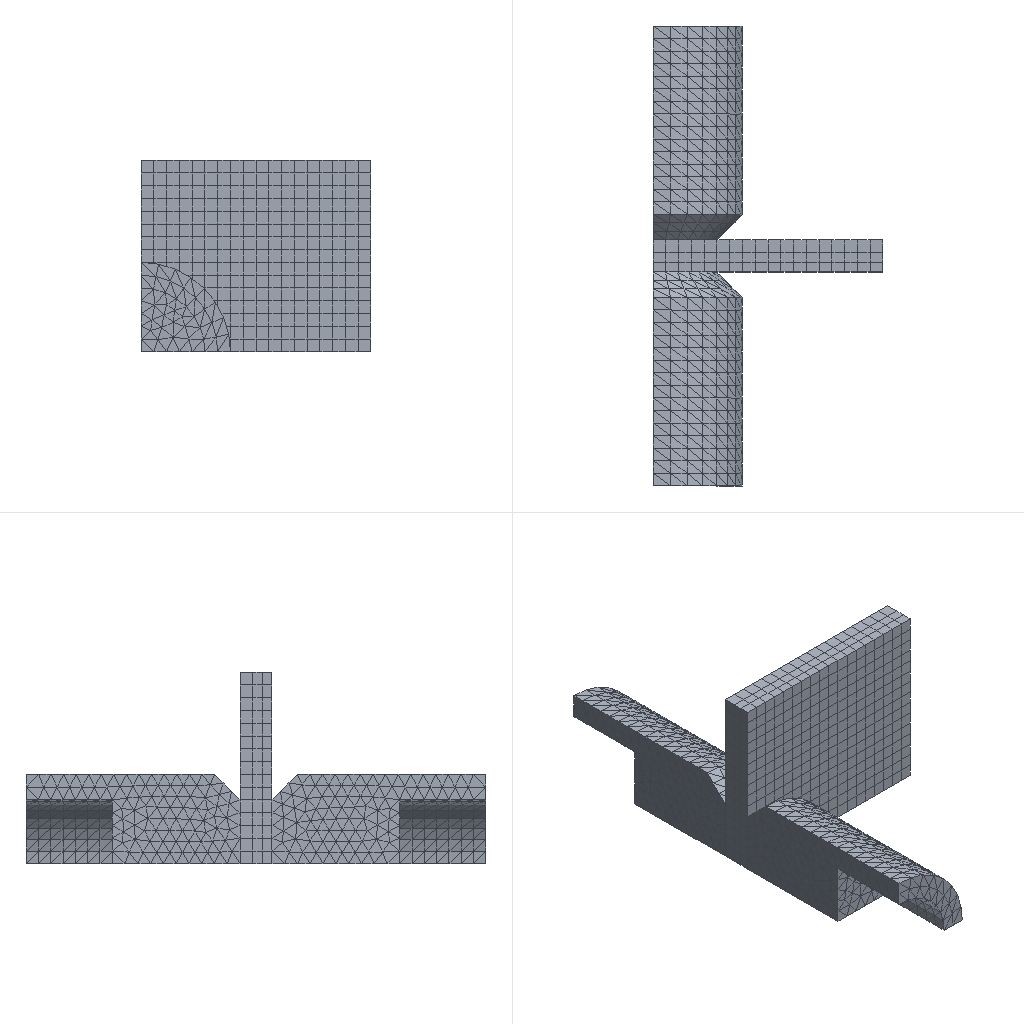Simulation study | abaqus
Set-up summary:
category,name,step,type,value,unit,region
solver,abaqus
solver,version,,,Abaqus/Standard 3DEXPERIENCE R2017x
units,not stated in the deck,,not stated
analysis,deck,,coupled temperature-displacement,coupled temperature-displacement
load_step,Step-1,Step-1,coupled temperature-displacement
load_step,requested,,,1
mesh,nodes,,,3054
mesh,elements,,,7094
element_type,Q3D4,,solid,6284
element_type,Q3D8,,solid,810
load,load commands in deck,,count,3
bc,support commands in deck,,count,5
material,BAN,,in results
material,DIANJI,,in results
check,setup vs results,,match,"per instance, exact: element labels, types and connectivity; labels of the nodes the elements use; coordinates of those nodes at SINGLE_PRECISION in 1 of 4 instance(s)"
Abaqus input file, long lists of numbers shortened:
*Heading
** Job name: Job-1 Model name: Model-1
** Generated by: Abaqus/CAE 2017
*Preprint, echo=NO, model=NO, history=NO, contact=NO
**
** PARTS
**
*Part, name=Part-1
*Node
      1,           0.,          10.,           5.
      2,           0.,        16.75,           5.
** (765 more lines like these left out)
*Element, type=Q3D4
   1, 440, 441, 442, 443
   2, 443, 444, 445, 446
** (3140 more lines like these left out)
*Nset, nset=Set-1, generate
   1,  767,    1
*Elset, elset=Set-1, generate
    1,  3142,     1
** Section: dianji
*Solid Section, elset=Set-1, material=dianji
,
*End Part
**
*Part, name=ban1
*Node
      1,           0.,          -1.,          15.
      2,           0.,           0.,          15.
** (606 more lines like these left out)
*Element, type=Q3D8
  1,  33,  34,  36,  35,   1,   2,   4,   3
  2,  35,  36,  38,  37,   3,   4,   6,   5
** (268 more lines like these left out)
*Nset, nset=Set-1, generate
   1,  608,    1
*Elset, elset=Set-1, generate
   1,  270,    1
** Section: ban
*Solid Section, elset=Set-1, material=ban
,
*End Part
**
*Part, name=ban1point5
*Node
      1,           0.,         -1.5,          15.
      2,           0.,        -0.75,          15.
** (910 more lines like these left out)
*Element, type=Q3D8
  1,  49,  50,  53,  52,   1,   2,   5,   4
  2,  50,  51,  54,  53,   2,   3,   6,   5
** (538 more lines like these left out)
*Nset, nset=Set-1, generate
   1,  912,    1
*Elset, elset=Set-1, generate
   1,  540,    1
** Section: ban
*Solid Section, elset=Set-1, material=ban
,
*End Part
**
**
** ASSEMBLY
**
*Assembly, name=Assembly
**
*Instance, name=Part-1-1, part=Part-1
          0.,           1.,           0.
*End Instance
**
*Instance, name=ban1-1, part=ban1
          0.,           1.,           0.
*End Instance
**
*Instance, name=ban1point5-1, part=ban1point5
*End Instance
**
*Instance, name=Part-1-2, part=Part-1
          0.,         -1.5,           0.
          0.,         -1.5,           0., 0.7071,         -1.5, 0.7071,         180.
*End Instance
**
*Nset, nset=Set-1, instance=Part-1-1, generate
   1,  767,    1
*Nset, nset=Set-1, instance=ban1-1, generate
   1,  608,    1
*Nset, nset=Set-1, instance=Part-1-2, generate
   1,  767,    1
*Nset, nset=Set-1, instance=ban1point5-1, generate
   1,  912,    1
*Elset, elset=Set-1, instance=Part-1-1, generate
    1,  3142,     1
*Elset, elset=Set-1, instance=ban1-1, generate
   1,  270,    1
*Elset, elset=Set-1, instance=Part-1-2, generate
    1,  3142,     1
*Elset, elset=Set-1, instance=ban1point5-1, generate
   1,  540,    1
*Nset, nset=Set-2, instance=Part-1-1
   3,   4,   6,   7,   9,  10,  11,  26,  27,  28,  29,  30,  31,  47,  52,  53
  54,  55,  77,  78,  79,  80,  81,  82,  83,  84,  85,  86,  87,  88,  89,  90
** (6 more lines like these left out)
*Nset, nset=Set-2, instance=ban1point5-1
  46,  47,  48,  94,  95,  96, 142, 143, 144, 190, 191, 192, 238, 239, 240, 286
 287, 288, 334, 335, 336, 382, 383, 384, 430, 431, 432, 478, 479, 480, 526, 527
** (2 more lines like these left out)
*Nset, nset=Set-2, instance=Part-1-2
   1,   2,   5,   7,   8,  10,  12,  13,  14,  15,  16,  17,  18,  39,  48,  49
  50,  51,  56,  57,  58,  59,  60,  61,  62,  63,  64,  65,  66,  67,  68,  69
** (6 more lines like these left out)
*Elset, elset=Set-2, instance=Part-1-1
  116,  177,  264,  308,  314,  315,  320,  363,  385,  387,  416,  469,  470,  471,  567,  570
  572,  573,  577,  593,  610,  628,  638,  657,  724,  725,  748,  755,  778,  785,  788,  801
** (10 more lines like these left out)
*Elset, elset=Set-2, instance=ban1point5-1
  29,  30,  59,  60,  89,  90, 119, 120, 149, 150, 179, 180, 209, 210, 239, 240
 269, 270, 299, 300, 329, 330, 359, 360, 389, 390, 419, 420, 449, 450, 479, 480
** (1 more lines like these left out)
*Elset, elset=Set-2, instance=Part-1-2
  315,  487,  536,  593,  598,  621,  622,  624,  632,  634,  635,  636,  637,  641,  643,  644
  653,  774,  796,  802,  908,  974,  992, 1022, 1123, 1154, 1191, 1193, 1223, 1229, 1233, 1249
** (10 more lines like these left out)
*Nset, nset=Set-3, instance=Part-1-1
   1,   2,   5,   7,   8,  10,  12,  13,  14,  15,  16,  17,  18,  39,  48,  49
  50,  51,  56,  57,  58,  59,  60,  61,  62,  63,  64,  65,  66,  67,  68,  69
** (6 more lines like these left out)
*Nset, nset=Set-3, instance=ban1point5-1, generate
  1,  48,   1
*Nset, nset=Set-3, instance=Part-1-2
   3,   4,   6,   7,   9,  10,  11,  26,  27,  28,  29,  30,  31,  47,  52,  53
  54,  55,  77,  78,  79,  80,  81,  82,  83,  84,  85,  86,  87,  88,  89,  90
** (6 more lines like these left out)
*Elset, elset=Set-3, instance=Part-1-1
  315,  487,  536,  593,  598,  621,  622,  624,  632,  634,  635,  636,  637,  641,  643,  644
  653,  774,  796,  802,  908,  974,  992, 1022, 1123, 1154, 1191, 1193, 1223, 1229, 1233, 1249
** (10 more lines like these left out)
*Elset, elset=Set-3, instance=ban1point5-1, generate
  1,  30,   1
*Elset, elset=Set-3, instance=Part-1-2
  116,  177,  264,  308,  314,  315,  320,  363,  385,  387,  416,  469,  470,  471,  567,  570
  572,  573,  577,  593,  610,  628,  638,  657,  724,  725,  748,  755,  778,  785,  788,  801
** (10 more lines like these left out)
*Nset, nset=Set-4, instance=Part-1-1
   2,   3,   5,   6,  19,  20,  21,  22,  23,  24,  25,  39,  40,  41,  42,  43
  44,  45,  46,  47, 161, 162, 163, 164, 165, 166, 167
*Elset, elset=Set-4, instance=Part-1-1
  277,  488,  757,  763,  764,  784, 1313, 1450, 1600, 1730, 1733, 1829, 1901, 1906, 1926, 2058
 2060, 2062, 2089, 2106, 2123, 2149, 2169, 2172, 2181, 2200, 2268, 2324, 2342, 2391, 2684, 2735
*Nset, nset=Set-5, instance=Part-1-1
   2,   3,   5,   6,  19,  20,  21,  22,  23,  24,  25,  39,  40,  41,  42,  43
  44,  45,  46,  47, 161, 162, 163, 164, 165, 166, 167
*Elset, elset=Set-5, instance=Part-1-1
  277,  488,  757,  763,  764,  784, 1313, 1450, 1600, 1730, 1733, 1829, 1901, 1906, 1926, 2058
 2060, 2062, 2089, 2106, 2123, 2149, 2169, 2172, 2181, 2200, 2268, 2324, 2342, 2391, 2684, 2735
*Elset, elset=_Surf-1_S1, internal, instance=ban1-1, generate
 256,  270,    1
*Elset, elset=_Surf-1_S1, internal, instance=ban1point5-1, generate
 511,  540,    1
*Elset, elset=_Surf-1_S6, internal, instance=ban1-1, generate
   1,  270,    1
*Elset, elset=_Surf-1_S6, internal, instance=ban1point5-1, generate
   1,  539,    2
*Elset, elset=_Surf-1_S2, internal, instance=ban1-1, generate
  1,  15,   1
*Elset, elset=_Surf-1_S2, internal, instance=ban1point5-1, generate
  1,  30,   1
*Elset, elset=_Surf-1_S4, internal, instance=ban1-1, generate
   1,  270,    1
*Elset, elset=_Surf-1_S4, internal, instance=ban1point5-1, generate
   2,  540,    2
*Elset, elset=_Surf-1_S3, internal, instance=ban1-1, generate
   1,  256,   15
*Elset, elset=_Surf-1_S3, internal, instance=ban1point5-1
   1,   2,  31,  32,  61,  62,  91,  92, 121, 122, 151, 152, 181, 182, 211, 212
 241, 242, 271, 272, 301, 302, 331, 332, 361, 362, 391, 392, 421, 422, 451, 452
** (1 more lines like these left out)
*Elset, elset=_Surf-1_S5, internal, instance=ban1-1, generate
  15,  270,   15
*Elset, elset=_Surf-1_S5, internal, instance=ban1point5-1
  29,  30,  59,  60,  89,  90, 119, 120, 149, 150, 179, 180, 209, 210, 239, 240
 269, 270, 299, 300, 329, 330, 359, 360, 389, 390, 419, 420, 449, 450, 479, 480
** (1 more lines like these left out)
*Surface, type=ELEMENT, name=Surf-1
_Surf-1_S1, S1
_Surf-1_S6, S6
_Surf-1_S2, S2
_Surf-1_S4, S4
_Surf-1_S3, S3
_Surf-1_S5, S5
*Elset, elset=_Surf-2_S3, internal, instance=Part-1-2
  277,  488,  757,  763,  764,  784, 1313, 1450, 1600, 1733, 1901, 1906, 2058, 2060, 2062, 2089
 2106, 2149, 2169, 2172, 2181, 2268, 2324, 2391, 2684, 2735
*Elset, elset=_Surf-2_S2, internal, instance=Part-1-2
 1730, 1926
*Elset, elset=_Surf-2_S4, internal, instance=Part-1-2
 1829, 2123
*Elset, elset=_Surf-2_S1, internal, instance=Part-1-2
 2200, 2342
*Surface, type=ELEMENT, name=Surf-2
_Surf-2_S3, S3
_Surf-2_S2, S2
_Surf-2_S4, S4
_Surf-2_S1, S1
*Elset, elset=_Surf-3_S3, internal, instance=Part-1-2
  113,  796, 1579, 1757, 1890, 1900, 1929, 1968, 1983, 2035, 2207, 2211, 2226, 2248, 2254, 2259
 2262, 2264, 2272, 2277, 2292, 2297, 2303, 2313, 2318, 2321, 2326, 2327, 2328, 2333, 2423, 2444
** (1 more lines like these left out)
*Elset, elset=_Surf-3_S4, internal, instance=Part-1-2
  315, 1863
*Surface, type=ELEMENT, name=Surf-3
_Surf-3_S3, S3
_Surf-3_S4, S4
*Elset, elset=_Surf-4_S3, internal, instance=Part-1-2
  277,  488,  757,  763,  764,  784, 1313, 1450, 1600, 1733, 1901, 1906, 2058, 2060, 2062, 2089
 2106, 2149, 2169, 2172, 2181, 2268, 2324, 2391, 2684, 2735
*Elset, elset=_Surf-4_S2, internal, instance=Part-1-2
 1730, 1926
*Elset, elset=_Surf-4_S4, internal, instance=Part-1-2
 1829, 2123
*Elset, elset=_Surf-4_S1, internal, instance=Part-1-2
 2200, 2342
*Surface, type=ELEMENT, name=Surf-4
_Surf-4_S3, S3
_Surf-4_S2, S2
_Surf-4_S4, S4
_Surf-4_S1, S1
*Elset, elset=_m_Surf-5_S4, internal, instance=Part-1-1
  270,  657, 2488
*Elset, elset=_m_Surf-5_S3, internal, instance=Part-1-1
  418, 1097, 1221, 1493, 1529, 1573, 1626, 2159, 2276, 2794, 2848, 2872, 2877, 2886, 2889, 2890
 2891, 2892, 2904, 2930, 2936, 2937, 2944, 2963, 2965, 2966, 2967, 2971, 2982, 2993, 2997, 3023
** (1 more lines like these left out)
*Elset, elset=_m_Surf-5_S1, internal, instance=Part-1-1
 2153, 3001
*Elset, elset=_m_Surf-5_S2, internal, instance=Part-1-1
 2843, 2973, 2978, 3108
*Surface, type=ELEMENT, name=m_Surf-5
_m_Surf-5_S4, S4
_m_Surf-5_S3, S3
_m_Surf-5_S2, S2
_m_Surf-5_S1, S1
*Elset, elset=_m_Surf-7_S6, internal, instance=ban1-1, generate
   1,  270,    1
*Surface, type=ELEMENT, name=m_Surf-7
_m_Surf-7_S6, S6
*Elset, elset=_m_Surf-9_S4, internal, instance=Part-1-2
  270,  657, 2488
*Elset, elset=_m_Surf-9_S3, internal, instance=Part-1-2
  418, 1097, 1221, 1493, 1529, 1573, 1626, 2159, 2276, 2794, 2848, 2872, 2877, 2886, 2889, 2890
 2891, 2892, 2904, 2930, 2936, 2937, 2944, 2963, 2965, 2966, 2967, 2971, 2982, 2993, 2997, 3023
** (1 more lines like these left out)
*Elset, elset=_m_Surf-9_S1, internal, instance=Part-1-2
 2153, 3001
*Elset, elset=_m_Surf-9_S2, internal, instance=Part-1-2
 2843, 2973, 2978, 3108
*Surface, type=ELEMENT, name=m_Surf-9
_m_Surf-9_S4, S4
_m_Surf-9_S3, S3
_m_Surf-9_S2, S2
_m_Surf-9_S1, S1
*Elset, elset=_s_Surf-5_S4, internal, instance=ban1-1, generate
   1,  270,    1
*Surface, type=ELEMENT, name=s_Surf-5
_s_Surf-5_S4, S4
*Elset, elset=_s_Surf-7_S4, internal, instance=ban1point5-1, generate
   2,  540,    2
*Surface, type=ELEMENT, name=s_Surf-7
_s_Surf-7_S4, S4
*Elset, elset=_s_Surf-9_S6, internal, instance=ban1point5-1, generate
   1,  539,    2
*Surface, type=ELEMENT, name=s_Surf-9
_s_Surf-9_S6, S6
** Constraint: Constraint-1
*Tie, name=Constraint-1, adjust=yes
s_Surf-5, m_Surf-5
** Constraint: Constraint-2
*Tie, name=Constraint-2, adjust=yes
m_Surf-7, s_Surf-7
** Constraint: Constraint-3
*Tie, name=Constraint-3, adjust=yes
s_Surf-9, m_Surf-9
*End Assembly
*Amplitude, name=Amp-1
             0.,              0.,           0.005,              1.
**
** MATERIALS
**
*Material, name=ban
*Conductivity
 7.2,
*Density
 7.18e-09,
*Elastic
80000., 0.3
*Electrical Conductivity
 0.523,
*Specific Heat
 4.77e+08,
*Material, name=dianji
*Conductivity
400.,
*Density
 8.9e-09,
*Elastic
110000., 0.34
*Electrical Conductivity
 5.9e+07,
*Specific Heat
 3.85e+08,
**
** PHYSICAL CONSTANTS
**
*Physical Constants, absolute zero=-273., stefan boltzmann=5.67e-08
**
** PREDEFINED FIELDS
**
** Name: Predefined Field-1   Type: Temperature
*Initial Conditions, type=TEMPERATURE
Set-1, 20.
** ----------------------------------------------------------------
**
** STEP: Step-1
**
*Step, name=Step-1, nlgeom=YES, inc=10000
*Coupled Temperature-displacement, electrical, creep=none, deltmx=100000., stabilize=0.0002, allsdtol=0.05, continue=NO
0.0001, 0.005, 5e-08, 0.005
**
** BOUNDARY CONDITIONS
**
** Name: BC-1 Type: 对称/反对称/完全固定
*Boundary
Set-2, ZSYMM
** Name: BC-2 Type: 对称/反对称/完全固定
*Boundary
Set-3, XSYMM
** Name: BC-3 Type: 位移/转角
*Boundary
Set-4, 2, 2
** Name: BC-4 Type: 电势
*Boundary
Set-5, 9, 9
**
** LOADS
**
** Name: Load-1   Type: Surface current
*Dsecurrent, amplitude=Amp-1
Surf-2,CS,410.
** Name: Load-2   Type: Pressure
*Dsload, amplitude=Amp-1
Surf-4, P, 0.05
**
** INTERACTIONS
**
** Interaction: Int-1
*Sfilm
Surf-1, F, 20., 5.
**
** OUTPUT REQUESTS
**
*Restart, write, frequency=0
**
** FIELD OUTPUT: F-Output-1
**
*Output, field
*Node Output
CECHG, CECUR, CF, EPOT, NT, RCHG, RECUR, RF
RFL, U
*Element Output, directions=YES
E, EFLX, EPG, HFL, LE, MISES, NCURS, PE, S, TEMP, VE, VEEQ, PEEQ
**
** HISTORY OUTPUT: H-Output-1
**
*Output, history, variable=PRESELECT
*End Step
Results summary:
result,step,,completed,increments=9 time=0.005/0.005
result,analysis,,,"coupled temperature-displacement, steady state"
result,last_loadstep,,,1
result,primary field,,,"U, NT11"
result,reaction total,,FX,-0.0,model units
result,reaction total,,FY,-0.9364,model units
result,reaction total,,FZ,-0.0,model units